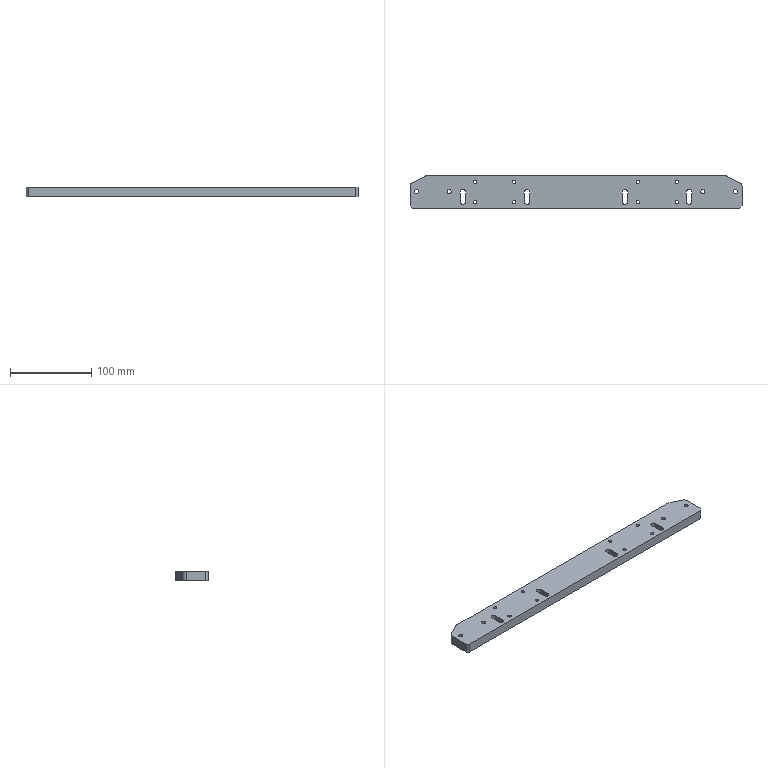Part | 1 solid | 62 faces | box 408 x 40 x 12 mm | volume 182666 mm3 | cylinder 32 | plane 30 | commonest cylinder face diameters 4.2 x8 6.6 x8 11 x8 5 x4 10 x4